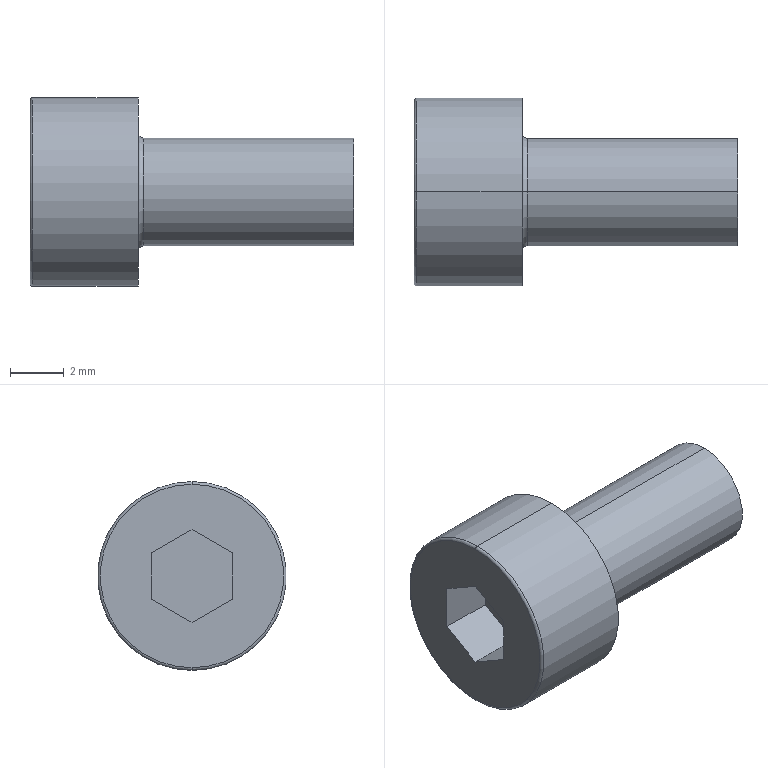Part | SolidWorks | features BlendCut 1, Cut 1, Fillet 1, LPattern 1, RevCut 1, Revolution 1 | 1 solid | 18 faces | box 12 x 7 x 7 mm | volume 239.16 mm3 | plane 10 | torus 4 | cylinder 4 | commonest cylinder face diameters 4 x2 7 x2
STEP:
#1=CARTESIAN_POINT('',(0.,0.,3.4));
#2=VERTEX_POINT('',#1);
#3=CARTESIAN_POINT('',(0.,0.,-3.4));
#4=VERTEX_POINT('',#3);
#5=CARTESIAN_POINT('',(0.,0.,0.));
#6=DIRECTION('',(-1.,0.,0.));
#7=DIRECTION('',(0.,0.,-1.));
#8=AXIS2_PLACEMENT_3D('',#5,#6,#7);
#9=CIRCLE('',#8,3.4);
#10=EDGE_CURVE('',#2,#4,#9,.T.);
#11=ORIENTED_EDGE('',*,*,#10,.F.);
#12=CARTESIAN_POINT('',(0.1,0.,3.5));
#13=VERTEX_POINT('',#12);
#14=CARTESIAN_POINT('',(0.1,0.,3.4));
#15=DIRECTION('',(0.,1.,0.));
#16=DIRECTION('',(0.,0.,1.));
#17=AXIS2_PLACEMENT_3D('',#14,#15,#16);
#18=CIRCLE('',#17,0.1);
#19=EDGE_CURVE('',#2,#13,#18,.T.);
#20=ORIENTED_EDGE('',*,*,#19,.T.);
#21=CARTESIAN_POINT('',(0.1,0.,-3.5));
#22=VERTEX_POINT('',#21);
#23=CARTESIAN_POINT('',(0.1,0.,0.));
#24=DIRECTION('',(1.,0.,0.));
#25=DIRECTION('',(0.,0.,-1.));
#26=AXIS2_PLACEMENT_3D('',#23,#24,#25);
#27=CIRCLE('',#26,3.5);
#28=EDGE_CURVE('',#22,#13,#27,.T.);
#29=ORIENTED_EDGE('',*,*,#28,.F.);
#30=CARTESIAN_POINT('',(0.1,0.,-3.4));
#31=DIRECTION('',(0.,-1.,0.));
#32=DIRECTION('',(0.,0.,-1.));
#33=AXIS2_PLACEMENT_3D('',#30,#31,#32);
#34=CIRCLE('',#33,0.1);
#35=EDGE_CURVE('',#4,#22,#34,.T.);
#36=ORIENTED_EDGE('',*,*,#35,.F.);
#37=EDGE_LOOP('',(#11,#20,#29,#36));
#38=FACE_OUTER_BOUND('',#37,.T.);
#39=CARTESIAN_POINT('',(0.1,0.,0.));
#40=DIRECTION('',(1.,0.,0.));
#41=DIRECTION('',(0.,0.,-1.));
#42=AXIS2_PLACEMENT_3D('',#39,#40,#41);
#43=TOROIDAL_SURFACE('',#42,3.4,0.1);
#44=ADVANCED_FACE('',(#38),#43,.T.);
#45=CARTESIAN_POINT('',(12.,0.,2.));
#46=VERTEX_POINT('',#45);
#47=CARTESIAN_POINT('',(12.,0.,-2.));
#48=VERTEX_POINT('',#47);
#49=CARTESIAN_POINT('',(12.,0.,0.));
#50=DIRECTION('',(-1.,0.,0.));
#51=DIRECTION('',(0.,0.,1.));
#52=AXIS2_PLACEMENT_3D('',#49,#50,#51);
#53=CIRCLE('',#52,2.);
#54=EDGE_CURVE('',#46,#48,#53,.T.);
#55=ORIENTED_EDGE('',*,*,#54,.T.);
#56=CARTESIAN_POINT('',(4.2,0.,-2.));
#57=VERTEX_POINT('',#56);
#58=CARTESIAN_POINT('',(0.,0.,-2.));
#59=DIRECTION('',(-1.,0.,0.));
#60=VECTOR('',#59,1000.);
#61=LINE('',#58,#60);
#62=EDGE_CURVE('',#48,#57,#61,.T.);
#63=ORIENTED_EDGE('',*,*,#62,.T.);
#64=CARTESIAN_POINT('',(4.2,0.,2.));
#65=VERTEX_POINT('',#64);
#66=CARTESIAN_POINT('',(4.2,0.,0.));
#67=DIRECTION('',(-1.,0.,0.));
#68=DIRECTION('',(0.,0.,1.));
#69=AXIS2_PLACEMENT_3D('',#66,#67,#68);
#70=CIRCLE('',#69,2.);
#71=EDGE_CURVE('',#65,#57,#70,.T.);
#72=ORIENTED_EDGE('',*,*,#71,.F.);
#73=CARTESIAN_POINT('',(0.,0.,2.));
#74=DIRECTION('',(-1.,0.,0.));
#75=VECTOR('',#74,1000.);
#76=LINE('',#73,#75);
#77=EDGE_CURVE('',#46,#65,#76,.T.);
#78=ORIENTED_EDGE('',*,*,#77,.F.);
#79=EDGE_LOOP('',(#55,#63,#72,#78));
#80=FACE_OUTER_BOUND('',#79,.T.);
#81=CARTESIAN_POINT('',(0.,0.,0.));
#82=DIRECTION('',(-1.,0.,0.));
#83=DIRECTION('',(0.,0.,1.));
#84=AXIS2_PLACEMENT_3D('',#81,#82,#83);
#85=CYLINDRICAL_SURFACE('',#84,2.);
#86=ADVANCED_FACE('',(#80),#85,.T.);
#87=CARTESIAN_POINT('',(4.,0.,-2.2));
#88=VERTEX_POINT('',#87);
#89=CARTESIAN_POINT('',(4.,0.,2.2));
#90=VERTEX_POINT('',#89);
#91=CARTESIAN_POINT('',(4.,0.,0.));
#92=DIRECTION('',(-1.,0.,0.));
#93=DIRECTION('',(0.,0.,1.));
#94=AXIS2_PLACEMENT_3D('',#91,#92,#93);
#95=CIRCLE('',#94,2.2);
#96=EDGE_CURVE('',#88,#90,#95,.T.);
#97=ORIENTED_EDGE('',*,*,#96,.F.);
#98=CARTESIAN_POINT('',(4.2,0.,-2.2));
#99=DIRECTION('',(0.,1.,0.));
#100=DIRECTION('',(0.,0.,1.));
#101=AXIS2_PLACEMENT_3D('',#98,#99,#100);
#102=CIRCLE('',#101,0.2);
#103=EDGE_CURVE('',#88,#57,#102,.T.);
#104=ORIENTED_EDGE('',*,*,#103,.T.);
#105=CARTESIAN_POINT('',(4.2,0.,0.));
#106=DIRECTION('',(-1.,0.,0.));
#107=DIRECTION('',(0.,0.,1.));
#108=AXIS2_PLACEMENT_3D('',#105,#106,#107);
#109=CIRCLE('',#108,2.);
#110=EDGE_CURVE('',#57,#65,#109,.T.);
#111=ORIENTED_EDGE('',*,*,#110,.T.);
#112=CARTESIAN_POINT('',(4.2,0.,2.2));
#113=DIRECTION('',(0.,-1.,0.));
#114=DIRECTION('',(0.,0.,-1.));
#115=AXIS2_PLACEMENT_3D('',#112,#113,#114);
#116=CIRCLE('',#115,0.2);
#117=EDGE_CURVE('',#90,#65,#116,.T.);
#118=ORIENTED_EDGE('',*,*,#117,.F.);
#119=EDGE_LOOP('',(#97,#104,#111,#118));
#120=FACE_OUTER_BOUND('',#119,.T.);
#121=CARTESIAN_POINT('',(4.2,0.,0.));
#122=DIRECTION('',(-1.,0.,0.));
#123=DIRECTION('',(0.,0.,1.));
#124=AXIS2_PLACEMENT_3D('',#121,#122,#123);
#125=TOROIDAL_SURFACE('',#124,2.2,0.2);
#126=ADVANCED_FACE('',(#120),#125,.F.);
#127=CARTESIAN_POINT('',(4.,0.,3.5));
#128=VERTEX_POINT('',#127);
#129=CARTESIAN_POINT('',(4.,0.,-3.5));
#130=VERTEX_POINT('',#129);
#131=CARTESIAN_POINT('',(4.,0.,0.));
#132=DIRECTION('',(-1.,0.,0.));
#133=DIRECTION('',(0.,0.,1.));
#134=AXIS2_PLACEMENT_3D('',#131,#132,#133);
#135=CIRCLE('',#134,3.5);
#136=EDGE_CURVE('',#128,#130,#135,.T.);
#137=ORIENTED_EDGE('',*,*,#136,.T.);
#138=CARTESIAN_POINT('',(0.,0.,-3.5));
#139=DIRECTION('',(-1.,0.,0.));
#140=VECTOR('',#139,1000.);
#141=LINE('',#138,#140);
#142=EDGE_CURVE('',#130,#22,#141,.T.);
#143=ORIENTED_EDGE('',*,*,#142,.T.);
#144=ORIENTED_EDGE('',*,*,#28,.T.);
#145=CARTESIAN_POINT('',(0.,0.,3.5));
#146=DIRECTION('',(-1.,0.,0.));
#147=VECTOR('',#146,1000.);
#148=LINE('',#145,#147);
#149=EDGE_CURVE('',#128,#13,#148,.T.);
#150=ORIENTED_EDGE('',*,*,#149,.F.);
#151=EDGE_LOOP('',(#137,#143,#144,#150));
#152=FACE_OUTER_BOUND('',#151,.T.);
#153=CARTESIAN_POINT('',(0.,0.,0.));
#154=DIRECTION('',(-1.,0.,0.));
#155=DIRECTION('',(0.,0.,1.));
#156=AXIS2_PLACEMENT_3D('',#153,#154,#155);
#157=CYLINDRICAL_SURFACE('',#156,3.5);
#158=ADVANCED_FACE('',(#152),#157,.T.);
#159=CARTESIAN_POINT('',(0.,0.,0.));
#160=DIRECTION('',(-1.,0.,0.));
#161=DIRECTION('',(0.,0.,-1.));
#162=AXIS2_PLACEMENT_3D('',#159,#160,#161);
#163=CIRCLE('',#162,3.4);
#164=EDGE_CURVE('',#4,#2,#163,.T.);
#165=ORIENTED_EDGE('',*,*,#164,.T.);
#166=ORIENTED_EDGE('',*,*,#10,.T.);
#167=EDGE_LOOP('',(#165,#166));
#168=FACE_OUTER_BOUND('',#167,.T.);
#169=CARTESIAN_POINT('',(0.,0.,1.72));
#170=VERTEX_POINT('',#169);
#171=CARTESIAN_POINT('',(0.,1.49,0.86));
#172=VERTEX_POINT('',#171);
#173=CARTESIAN_POINT('',(0.,0.,1.72));
#174=DIRECTION('',(0.,0.866,-0.5));
#175=VECTOR('',#174,1000.);
#176=LINE('',#173,#175);
#177=EDGE_CURVE('',#170,#172,#176,.T.);
#178=ORIENTED_EDGE('',*,*,#177,.F.);
#179=CARTESIAN_POINT('',(0.,-1.49,0.86));
#180=VERTEX_POINT('',#179);
#181=CARTESIAN_POINT('',(0.,-1.49,0.86));
#182=DIRECTION('',(0.,0.866,0.5));
#183=VECTOR('',#182,1000.);
#184=LINE('',#181,#183);
#185=EDGE_CURVE('',#180,#170,#184,.T.);
#186=ORIENTED_EDGE('',*,*,#185,.F.);
#187=CARTESIAN_POINT('',(0.,-1.49,-0.86));
#188=VERTEX_POINT('',#187);
#189=CARTESIAN_POINT('',(0.,-1.49,-0.86));
#190=DIRECTION('',(0.,0.,1.));
#191=VECTOR('',#190,1000.);
#192=LINE('',#189,#191);
#193=EDGE_CURVE('',#188,#180,#192,.T.);
#194=ORIENTED_EDGE('',*,*,#193,.F.);
#195=CARTESIAN_POINT('',(0.,0.,-1.72));
#196=VERTEX_POINT('',#195);
#197=CARTESIAN_POINT('',(0.,0.,-1.72));
#198=DIRECTION('',(0.,-0.866,0.5));
#199=VECTOR('',#198,1000.);
#200=LINE('',#197,#199);
#201=EDGE_CURVE('',#196,#188,#200,.T.);
#202=ORIENTED_EDGE('',*,*,#201,.F.);
#203=CARTESIAN_POINT('',(0.,1.49,-0.86));
#204=VERTEX_POINT('',#203);
#205=CARTESIAN_POINT('',(0.,1.49,-0.86));
#206=DIRECTION('',(0.,-0.866,-0.5));
#207=VECTOR('',#206,1000.);
#208=LINE('',#205,#207);
#209=EDGE_CURVE('',#204,#196,#208,.T.);
#210=ORIENTED_EDGE('',*,*,#209,.F.);
#211=CARTESIAN_POINT('',(0.,1.49,0.86));
#212=DIRECTION('',(0.,0.,-1.));
#213=VECTOR('',#212,1000.);
#214=LINE('',#211,#213);
#215=EDGE_CURVE('',#172,#204,#214,.T.);
#216=ORIENTED_EDGE('',*,*,#215,.F.);
#217=EDGE_LOOP('',(#178,#186,#194,#202,#210,#216));
#218=FACE_BOUND('',#217,.T.);
#219=CARTESIAN_POINT('',(0.,0.,0.));
#220=DIRECTION('',(1.,0.,0.));
#221=DIRECTION('',(0.,0.,-1.));
#222=AXIS2_PLACEMENT_3D('',#219,#220,#221);
#223=PLANE('',#222);
#224=ADVANCED_FACE('',(#168,#218),#223,.F.);
#225=ORIENTED_EDGE('',*,*,#142,.F.);
#226=CARTESIAN_POINT('',(4.,0.,0.));
#227=DIRECTION('',(-1.,0.,0.));
#228=DIRECTION('',(0.,0.,1.));
#229=AXIS2_PLACEMENT_3D('',#226,#227,#228);
#230=CIRCLE('',#229,3.5);
#231=EDGE_CURVE('',#130,#128,#230,.T.);
#232=ORIENTED_EDGE('',*,*,#231,.T.);
#233=ORIENTED_EDGE('',*,*,#149,.T.);
#234=CARTESIAN_POINT('',(0.1,0.,0.));
#235=DIRECTION('',(1.,0.,0.));
#236=DIRECTION('',(0.,0.,-1.));
#237=AXIS2_PLACEMENT_3D('',#234,#235,#236);
#238=CIRCLE('',#237,3.5);
#239=EDGE_CURVE('',#13,#22,#238,.T.);
#240=ORIENTED_EDGE('',*,*,#239,.T.);
#241=EDGE_LOOP('',(#225,#232,#233,#240));
#242=FACE_OUTER_BOUND('',#241,.T.);
#243=CARTESIAN_POINT('',(0.,0.,0.));
#244=DIRECTION('',(-1.,0.,0.));
#245=DIRECTION('',(0.,0.,1.));
#246=AXIS2_PLACEMENT_3D('',#243,#244,#245);
#247=CYLINDRICAL_SURFACE('',#246,3.5);
#248=ADVANCED_FACE('',(#242),#247,.T.);
#249=ORIENTED_EDGE('',*,*,#136,.F.);
#250=ORIENTED_EDGE('',*,*,#231,.F.);
#251=EDGE_LOOP('',(#249,#250));
#252=FACE_OUTER_BOUND('',#251,.T.);
#253=CARTESIAN_POINT('',(4.,0.,0.));
#254=DIRECTION('',(-1.,0.,0.));
#255=DIRECTION('',(0.,0.,1.));
#256=AXIS2_PLACEMENT_3D('',#253,#254,#255);
#257=CIRCLE('',#256,2.2);
#258=EDGE_CURVE('',#90,#88,#257,.T.);
#259=ORIENTED_EDGE('',*,*,#258,.T.);
#260=ORIENTED_EDGE('',*,*,#96,.T.);
#261=EDGE_LOOP('',(#259,#260));
#262=FACE_BOUND('',#261,.T.);
#263=CARTESIAN_POINT('',(4.,3.5,0.));
#264=DIRECTION('',(-1.,0.,0.));
#265=DIRECTION('',(0.,0.,1.));
#266=AXIS2_PLACEMENT_3D('',#263,#264,#265);
#267=PLANE('',#266);
#268=ADVANCED_FACE('',(#252,#262),#267,.F.);
#269=ORIENTED_EDGE('',*,*,#103,.F.);
#270=ORIENTED_EDGE('',*,*,#258,.F.);
#271=ORIENTED_EDGE('',*,*,#117,.T.);
#272=ORIENTED_EDGE('',*,*,#71,.T.);
#273=EDGE_LOOP('',(#269,#270,#271,#272));
#274=FACE_OUTER_BOUND('',#273,.T.);
#275=CARTESIAN_POINT('',(4.2,0.,0.));
#276=DIRECTION('',(-1.,0.,0.));
#277=DIRECTION('',(0.,0.,1.));
#278=AXIS2_PLACEMENT_3D('',#275,#276,#277);
#279=TOROIDAL_SURFACE('',#278,2.2,0.2);
#280=ADVANCED_FACE('',(#274),#279,.F.);
#281=ORIENTED_EDGE('',*,*,#62,.F.);
#282=CARTESIAN_POINT('',(12.,0.,0.));
#283=DIRECTION('',(-1.,0.,0.));
#284=DIRECTION('',(0.,0.,1.));
#285=AXIS2_PLACEMENT_3D('',#282,#283,#284);
#286=CIRCLE('',#285,2.);
#287=EDGE_CURVE('',#48,#46,#286,.T.);
#288=ORIENTED_EDGE('',*,*,#287,.T.);
#289=ORIENTED_EDGE('',*,*,#77,.T.);
#290=ORIENTED_EDGE('',*,*,#110,.F.);
#291=EDGE_LOOP('',(#281,#288,#289,#290));
#292=FACE_OUTER_BOUND('',#291,.T.);
#293=CARTESIAN_POINT('',(0.,0.,0.));
#294=DIRECTION('',(-1.,0.,0.));
#295=DIRECTION('',(0.,0.,1.));
#296=AXIS2_PLACEMENT_3D('',#293,#294,#295);
#297=CYLINDRICAL_SURFACE('',#296,2.);
#298=ADVANCED_FACE('',(#292),#297,.T.);
#299=ORIENTED_EDGE('',*,*,#54,.F.);
#300=ORIENTED_EDGE('',*,*,#287,.F.);
#301=EDGE_LOOP('',(#299,#300));
#302=FACE_OUTER_BOUND('',#301,.T.);
#303=CARTESIAN_POINT('',(12.,2.,0.));
#304=DIRECTION('',(-1.,0.,0.));
#305=DIRECTION('',(0.,0.,1.));
#306=AXIS2_PLACEMENT_3D('',#303,#304,#305);
#307=PLANE('',#306);
#308=ADVANCED_FACE('',(#302),#307,.F.);
#309=ORIENTED_EDGE('',*,*,#185,.T.);
#310=CARTESIAN_POINT('',(2.,0.,1.72));
#311=VERTEX_POINT('',#310);
#312=CARTESIAN_POINT('',(2.,0.,1.72));
#313=DIRECTION('',(-1.,0.,0.));
#314=VECTOR('',#313,1000.);
#315=LINE('',#312,#314);
#316=EDGE_CURVE('',#311,#170,#315,.T.);
#317=ORIENTED_EDGE('',*,*,#316,.F.);
#318=CARTESIAN_POINT('',(2.,-1.49,0.86));
#319=VERTEX_POINT('',#318);
#320=CARTESIAN_POINT('',(2.,-1.49,0.86));
#321=DIRECTION('',(0.,0.866,0.5));
#322=VECTOR('',#321,1000.);
#323=LINE('',#320,#322);
#324=EDGE_CURVE('',#319,#311,#323,.T.);
#325=ORIENTED_EDGE('',*,*,#324,.F.);
#326=CARTESIAN_POINT('',(2.,-1.49,0.86));
#327=DIRECTION('',(-1.,0.,0.));
#328=VECTOR('',#327,1000.);
#329=LINE('',#326,#328);
#330=EDGE_CURVE('',#319,#180,#329,.T.);
#331=ORIENTED_EDGE('',*,*,#330,.T.);
#332=EDGE_LOOP('',(#309,#317,#325,#331));
#333=FACE_OUTER_BOUND('',#332,.T.);
#334=CARTESIAN_POINT('',(2.,-1.49,0.86));
#335=DIRECTION('',(0.,-0.5,0.866));
#336=DIRECTION('',(0.,-0.866,-0.5));
#337=AXIS2_PLACEMENT_3D('',#334,#335,#336);
#338=PLANE('',#337);
#339=ADVANCED_FACE('',(#333),#338,.F.);
#340=ORIENTED_EDGE('',*,*,#193,.T.);
#341=ORIENTED_EDGE('',*,*,#330,.F.);
#342=CARTESIAN_POINT('',(2.,-1.49,-0.86));
#343=VERTEX_POINT('',#342);
#344=CARTESIAN_POINT('',(2.,-1.49,-0.86));
#345=DIRECTION('',(0.,0.,1.));
#346=VECTOR('',#345,1000.);
#347=LINE('',#344,#346);
#348=EDGE_CURVE('',#343,#319,#347,.T.);
#349=ORIENTED_EDGE('',*,*,#348,.F.);
#350=CARTESIAN_POINT('',(2.,-1.49,-0.86));
#351=DIRECTION('',(-1.,0.,0.));
#352=VECTOR('',#351,1000.);
#353=LINE('',#350,#352);
#354=EDGE_CURVE('',#343,#188,#353,.T.);
#355=ORIENTED_EDGE('',*,*,#354,.T.);
#356=EDGE_LOOP('',(#340,#341,#349,#355));
#357=FACE_OUTER_BOUND('',#356,.T.);
#358=CARTESIAN_POINT('',(2.,-1.49,-0.86));
#359=DIRECTION('',(0.,-1.,0.));
#360=DIRECTION('',(0.,0.,-1.));
#361=AXIS2_PLACEMENT_3D('',#358,#359,#360);
#362=PLANE('',#361);
#363=ADVANCED_FACE('',(#357),#362,.F.);
#364=ORIENTED_EDGE('',*,*,#201,.T.);
#365=ORIENTED_EDGE('',*,*,#354,.F.);
#366=CARTESIAN_POINT('',(2.,0.,-1.72));
#367=VERTEX_POINT('',#366);
#368=CARTESIAN_POINT('',(2.,0.,-1.72));
#369=DIRECTION('',(0.,-0.866,0.5));
#370=VECTOR('',#369,1000.);
#371=LINE('',#368,#370);
#372=EDGE_CURVE('',#367,#343,#371,.T.);
#373=ORIENTED_EDGE('',*,*,#372,.F.);
#374=CARTESIAN_POINT('',(2.,0.,-1.72));
#375=DIRECTION('',(-1.,0.,0.));
#376=VECTOR('',#375,1000.);
#377=LINE('',#374,#376);
#378=EDGE_CURVE('',#367,#196,#377,.T.);
#379=ORIENTED_EDGE('',*,*,#378,.T.);
#380=EDGE_LOOP('',(#364,#365,#373,#379));
#381=FACE_OUTER_BOUND('',#380,.T.);
#382=CARTESIAN_POINT('',(2.,0.,-1.72));
#383=DIRECTION('',(0.,-0.5,-0.866));
#384=DIRECTION('',(0.,0.866,-0.5));
#385=AXIS2_PLACEMENT_3D('',#382,#383,#384);
#386=PLANE('',#385);
#387=ADVANCED_FACE('',(#381),#386,.F.);
#388=ORIENTED_EDGE('',*,*,#209,.T.);
#389=ORIENTED_EDGE('',*,*,#378,.F.);
#390=CARTESIAN_POINT('',(2.,1.49,-0.86));
#391=VERTEX_POINT('',#390);
#392=CARTESIAN_POINT('',(2.,1.49,-0.86));
#393=DIRECTION('',(0.,-0.866,-0.5));
#394=VECTOR('',#393,1000.);
#395=LINE('',#392,#394);
#396=EDGE_CURVE('',#391,#367,#395,.T.);
#397=ORIENTED_EDGE('',*,*,#396,.F.);
#398=CARTESIAN_POINT('',(2.,1.49,-0.86));
#399=DIRECTION('',(-1.,0.,0.));
#400=VECTOR('',#399,1000.);
#401=LINE('',#398,#400);
#402=EDGE_CURVE('',#391,#204,#401,.T.);
#403=ORIENTED_EDGE('',*,*,#402,.T.);
#404=EDGE_LOOP('',(#388,#389,#397,#403));
#405=FACE_OUTER_BOUND('',#404,.T.);
#406=CARTESIAN_POINT('',(2.,1.49,-0.86));
#407=DIRECTION('',(0.,0.5,-0.866));
#408=DIRECTION('',(0.,0.866,0.5));
#409=AXIS2_PLACEMENT_3D('',#406,#407,#408);
#410=PLANE('',#409);
#411=ADVANCED_FACE('',(#405),#410,.F.);
#412=ORIENTED_EDGE('',*,*,#215,.T.);
#413=ORIENTED_EDGE('',*,*,#402,.F.);
#414=CARTESIAN_POINT('',(2.,1.49,0.86));
#415=VERTEX_POINT('',#414);
#416=CARTESIAN_POINT('',(2.,1.49,0.86));
#417=DIRECTION('',(0.,0.,-1.));
#418=VECTOR('',#417,1000.);
#419=LINE('',#416,#418);
#420=EDGE_CURVE('',#415,#391,#419,.T.);
#421=ORIENTED_EDGE('',*,*,#420,.F.);
#422=CARTESIAN_POINT('',(2.,1.49,0.86));
#423=DIRECTION('',(-1.,0.,0.));
#424=VECTOR('',#423,1000.);
#425=LINE('',#422,#424);
#426=EDGE_CURVE('',#415,#172,#425,.T.);
#427=ORIENTED_EDGE('',*,*,#426,.T.);
#428=EDGE_LOOP('',(#412,#413,#421,#427));
#429=FACE_OUTER_BOUND('',#428,.T.);
#430=CARTESIAN_POINT('',(2.,1.49,0.86));
#431=DIRECTION('',(0.,1.,0.));
#432=DIRECTION('',(0.,0.,1.));
#433=AXIS2_PLACEMENT_3D('',#430,#431,#432);
#434=PLANE('',#433);
#435=ADVANCED_FACE('',(#429),#434,.F.);
#436=ORIENTED_EDGE('',*,*,#177,.T.);
#437=ORIENTED_EDGE('',*,*,#426,.F.);
#438=CARTESIAN_POINT('',(2.,0.,1.72));
#439=DIRECTION('',(0.,0.866,-0.5));
#440=VECTOR('',#439,1000.);
#441=LINE('',#438,#440);
#442=EDGE_CURVE('',#311,#415,#441,.T.);
#443=ORIENTED_EDGE('',*,*,#442,.F.);
#444=ORIENTED_EDGE('',*,*,#316,.T.);
#445=EDGE_LOOP('',(#436,#437,#443,#444));
#446=FACE_OUTER_BOUND('',#445,.T.);
#447=CARTESIAN_POINT('',(2.,0.,1.72));
#448=DIRECTION('',(0.,0.5,0.866));
#449=DIRECTION('',(0.,-0.866,0.5));
#450=AXIS2_PLACEMENT_3D('',#447,#448,#449);
#451=PLANE('',#450);
#452=ADVANCED_FACE('',(#446),#451,.F.);
#453=ORIENTED_EDGE('',*,*,#324,.T.);
#454=ORIENTED_EDGE('',*,*,#442,.T.);
#455=ORIENTED_EDGE('',*,*,#420,.T.);
#456=ORIENTED_EDGE('',*,*,#396,.T.);
#457=ORIENTED_EDGE('',*,*,#372,.T.);
#458=ORIENTED_EDGE('',*,*,#348,.T.);
#459=EDGE_LOOP('',(#453,#454,#455,#456,#457,#458));
#460=FACE_OUTER_BOUND('',#459,.T.);
#461=CARTESIAN_POINT('',(2.,1.49,2.58));
#462=DIRECTION('',(-1.,0.,0.));
#463=DIRECTION('',(0.,0.,1.));
#464=AXIS2_PLACEMENT_3D('',#461,#462,#463);
#465=PLANE('',#464);
#466=ADVANCED_FACE('',(#460),#465,.T.);
#467=ORIENTED_EDGE('',*,*,#19,.F.);
#468=ORIENTED_EDGE('',*,*,#164,.F.);
#469=ORIENTED_EDGE('',*,*,#35,.T.);
#470=ORIENTED_EDGE('',*,*,#239,.F.);
#471=EDGE_LOOP('',(#467,#468,#469,#470));
#472=FACE_OUTER_BOUND('',#471,.T.);
#473=CARTESIAN_POINT('',(0.1,0.,0.));
#474=DIRECTION('',(1.,0.,0.));
#475=DIRECTION('',(0.,0.,-1.));
#476=AXIS2_PLACEMENT_3D('',#473,#474,#475);
#477=TOROIDAL_SURFACE('',#476,3.4,0.1);
#478=ADVANCED_FACE('',(#472),#477,.T.);
#479=CLOSED_SHELL('',(#44,#86,#126,#158,#224,#248,#268,#280,#298,#308,#339,#363,#387,#411,#435,#452,#466,#478));
#480=MANIFOLD_SOLID_BREP('',#479);
#481=CARTESIAN_POINT('',(0.,0.,0.));
#482=DIRECTION('',(0.,0.,1.));
#483=DIRECTION('',(1.,0.,0.));
#484=AXIS2_PLACEMENT_3D('',#481,#482,#483);
#485=(LENGTH_UNIT()NAMED_UNIT(*)SI_UNIT(.MILLI.,.METRE.));
#486=UNCERTAINTY_MEASURE_WITH_UNIT(LENGTH_MEASURE(0.00001),#485,'','');
#487=(NAMED_UNIT(*)PLANE_ANGLE_UNIT()SI_UNIT($,.RADIAN.));
#488=(NAMED_UNIT(*)SI_UNIT($,.STERADIAN.)SOLID_ANGLE_UNIT());
#489=(GEOMETRIC_REPRESENTATION_CONTEXT(3)GLOBAL_UNCERTAINTY_ASSIGNED_CONTEXT((#486))GLOBAL_UNIT_ASSIGNED_CONTEXT((#485,#487,#488))REPRESENTATION_CONTEXT('',''));
#490=ADVANCED_BREP_SHAPE_REPRESENTATION('',(#480,#484),#489);